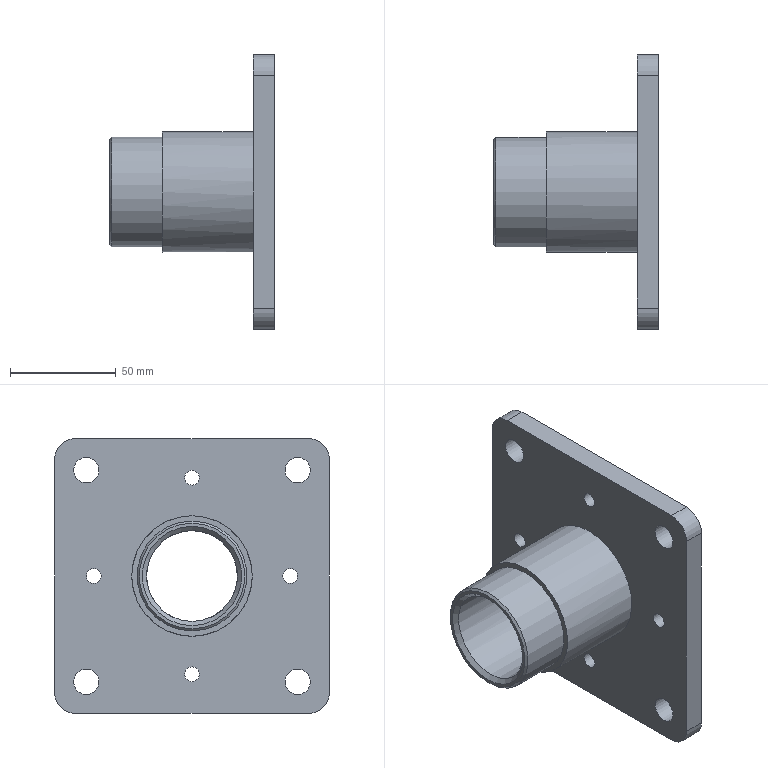Part | STEP file | HL4GZ-1.581.029 (hydraulic tank outlet front flange) | 2 solids | 31 faces | box 78 x 130 x 130 mm | volume 210630 mm3 | cylinder 17 | plane 11 | cone 3 | commonest cylinder face diameters 7 x4 12 x4 20 x4 52 x3 43 x1 57 x1